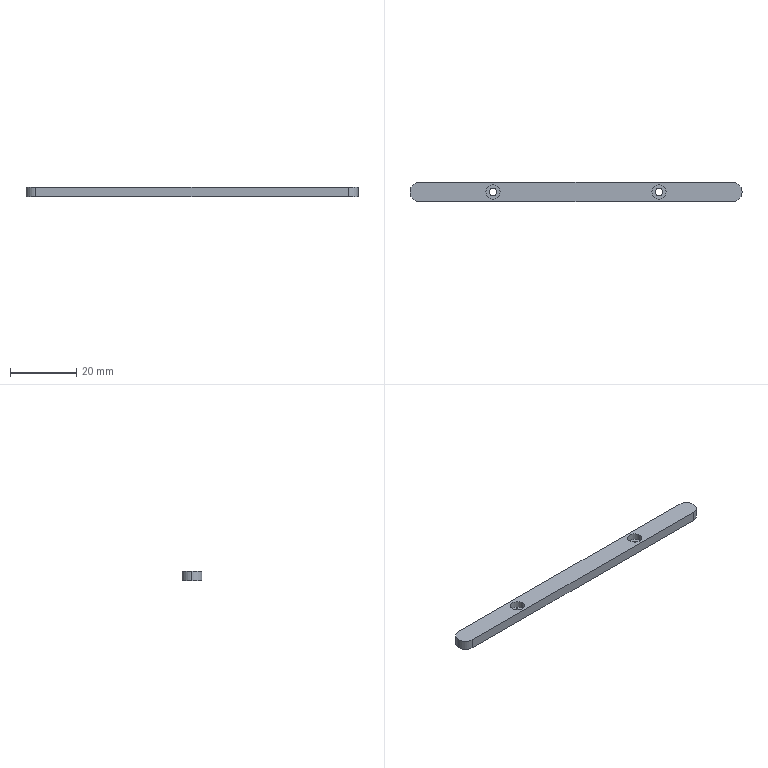Part | SolidWorks | features 3DProfileFeature 1, Extrusion 1, Fillet 1, HoleWzd 1 | 1 solid | 18 faces | box 100 x 6 x 3 mm | volume 1710 mm3 | cylinder 12 | plane 6 | commonest cylinder face diameters 2.4 x4 4.3 x4 6 x4
STEP:
#1=CARTESIAN_POINT('',(-27.15,-40.35,1.));
#2=VERTEX_POINT('',#1);
#3=CARTESIAN_POINT('',(-22.85,-40.35,1.));
#4=VERTEX_POINT('',#3);
#5=CARTESIAN_POINT('',(-25.,-40.35,1.));
#6=DIRECTION('',(0.,0.,1.));
#7=DIRECTION('',(1.,0.,0.));
#8=AXIS2_PLACEMENT_3D('',#5,#6,#7);
#9=CIRCLE('',#8,2.15);
#10=EDGE_CURVE('',#2,#4,#9,.T.);
#11=ORIENTED_EDGE('',*,*,#10,.F.);
#12=CARTESIAN_POINT('',(-27.15,-40.35,3.));
#13=VERTEX_POINT('',#12);
#14=CARTESIAN_POINT('',(-27.15,-40.35,3.));
#15=DIRECTION('',(0.,0.,1.));
#16=VECTOR('',#15,1000.);
#17=LINE('',#14,#16);
#18=EDGE_CURVE('',#2,#13,#17,.T.);
#19=ORIENTED_EDGE('',*,*,#18,.T.);
#20=CARTESIAN_POINT('',(-22.85,-40.35,3.));
#21=VERTEX_POINT('',#20);
#22=CARTESIAN_POINT('',(-25.,-40.35,3.));
#23=DIRECTION('',(0.,0.,1.));
#24=DIRECTION('',(1.,0.,0.));
#25=AXIS2_PLACEMENT_3D('',#22,#23,#24);
#26=CIRCLE('',#25,2.15);
#27=EDGE_CURVE('',#13,#21,#26,.T.);
#28=ORIENTED_EDGE('',*,*,#27,.T.);
#29=CARTESIAN_POINT('',(-22.85,-40.35,3.));
#30=DIRECTION('',(0.,0.,1.));
#31=VECTOR('',#30,1000.);
#32=LINE('',#29,#31);
#33=EDGE_CURVE('',#4,#21,#32,.T.);
#34=ORIENTED_EDGE('',*,*,#33,.F.);
#35=EDGE_LOOP('',(#11,#19,#28,#34));
#36=FACE_OUTER_BOUND('',#35,.T.);
#37=CARTESIAN_POINT('',(-25.,-40.35,3.));
#38=DIRECTION('',(0.,0.,1.));
#39=DIRECTION('',(1.,0.,0.));
#40=AXIS2_PLACEMENT_3D('',#37,#38,#39);
#41=CYLINDRICAL_SURFACE('',#40,2.15);
#42=ADVANCED_FACE('',(#36),#41,.F.);
#43=CARTESIAN_POINT('',(-26.2,-40.35,0.));
#44=VERTEX_POINT('',#43);
#45=CARTESIAN_POINT('',(-23.8,-40.35,0.));
#46=VERTEX_POINT('',#45);
#47=CARTESIAN_POINT('',(-25.,-40.35,0.));
#48=DIRECTION('',(0.,0.,1.));
#49=DIRECTION('',(1.,0.,0.));
#50=AXIS2_PLACEMENT_3D('',#47,#48,#49);
#51=CIRCLE('',#50,1.2);
#52=EDGE_CURVE('',#44,#46,#51,.T.);
#53=ORIENTED_EDGE('',*,*,#52,.F.);
#54=CARTESIAN_POINT('',(-26.2,-40.35,1.));
#55=VERTEX_POINT('',#54);
#56=CARTESIAN_POINT('',(-26.2,-40.35,3.));
#57=DIRECTION('',(0.,0.,1.));
#58=VECTOR('',#57,1000.);
#59=LINE('',#56,#58);
#60=EDGE_CURVE('',#44,#55,#59,.T.);
#61=ORIENTED_EDGE('',*,*,#60,.T.);
#62=CARTESIAN_POINT('',(-23.8,-40.35,1.));
#63=VERTEX_POINT('',#62);
#64=CARTESIAN_POINT('',(-25.,-40.35,1.));
#65=DIRECTION('',(0.,0.,1.));
#66=DIRECTION('',(1.,0.,0.));
#67=AXIS2_PLACEMENT_3D('',#64,#65,#66);
#68=CIRCLE('',#67,1.2);
#69=EDGE_CURVE('',#55,#63,#68,.T.);
#70=ORIENTED_EDGE('',*,*,#69,.T.);
#71=CARTESIAN_POINT('',(-23.8,-40.35,3.));
#72=DIRECTION('',(0.,0.,1.));
#73=VECTOR('',#72,1000.);
#74=LINE('',#71,#73);
#75=EDGE_CURVE('',#46,#63,#74,.T.);
#76=ORIENTED_EDGE('',*,*,#75,.F.);
#77=EDGE_LOOP('',(#53,#61,#70,#76));
#78=FACE_OUTER_BOUND('',#77,.T.);
#79=CARTESIAN_POINT('',(-25.,-40.35,3.));
#80=DIRECTION('',(0.,0.,1.));
#81=DIRECTION('',(1.,0.,0.));
#82=AXIS2_PLACEMENT_3D('',#79,#80,#81);
#83=CYLINDRICAL_SURFACE('',#82,1.2);
#84=ADVANCED_FACE('',(#78),#83,.F.);
#85=CARTESIAN_POINT('',(22.85,-40.35,1.));
#86=VERTEX_POINT('',#85);
#87=CARTESIAN_POINT('',(27.15,-40.35,1.));
#88=VERTEX_POINT('',#87);
#89=CARTESIAN_POINT('',(25.,-40.35,1.));
#90=DIRECTION('',(0.,0.,1.));
#91=DIRECTION('',(1.,0.,0.));
#92=AXIS2_PLACEMENT_3D('',#89,#90,#91);
#93=CIRCLE('',#92,2.15);
#94=EDGE_CURVE('',#86,#88,#93,.T.);
#95=ORIENTED_EDGE('',*,*,#94,.F.);
#96=CARTESIAN_POINT('',(22.85,-40.35,3.));
#97=VERTEX_POINT('',#96);
#98=CARTESIAN_POINT('',(22.85,-40.35,3.));
#99=DIRECTION('',(0.,0.,1.));
#100=VECTOR('',#99,1000.);
#101=LINE('',#98,#100);
#102=EDGE_CURVE('',#86,#97,#101,.T.);
#103=ORIENTED_EDGE('',*,*,#102,.T.);
#104=CARTESIAN_POINT('',(27.15,-40.35,3.));
#105=VERTEX_POINT('',#104);
#106=CARTESIAN_POINT('',(25.,-40.35,3.));
#107=DIRECTION('',(0.,0.,1.));
#108=DIRECTION('',(1.,0.,0.));
#109=AXIS2_PLACEMENT_3D('',#106,#107,#108);
#110=CIRCLE('',#109,2.15);
#111=EDGE_CURVE('',#97,#105,#110,.T.);
#112=ORIENTED_EDGE('',*,*,#111,.T.);
#113=CARTESIAN_POINT('',(27.15,-40.35,3.));
#114=DIRECTION('',(0.,0.,1.));
#115=VECTOR('',#114,1000.);
#116=LINE('',#113,#115);
#117=EDGE_CURVE('',#88,#105,#116,.T.);
#118=ORIENTED_EDGE('',*,*,#117,.F.);
#119=EDGE_LOOP('',(#95,#103,#112,#118));
#120=FACE_OUTER_BOUND('',#119,.T.);
#121=CARTESIAN_POINT('',(25.,-40.35,3.));
#122=DIRECTION('',(0.,0.,1.));
#123=DIRECTION('',(1.,0.,0.));
#124=AXIS2_PLACEMENT_3D('',#121,#122,#123);
#125=CYLINDRICAL_SURFACE('',#124,2.15);
#126=ADVANCED_FACE('',(#120),#125,.F.);
#127=CARTESIAN_POINT('',(23.8,-40.35,0.));
#128=VERTEX_POINT('',#127);
#129=CARTESIAN_POINT('',(26.2,-40.35,0.));
#130=VERTEX_POINT('',#129);
#131=CARTESIAN_POINT('',(25.,-40.35,0.));
#132=DIRECTION('',(0.,0.,1.));
#133=DIRECTION('',(1.,0.,0.));
#134=AXIS2_PLACEMENT_3D('',#131,#132,#133);
#135=CIRCLE('',#134,1.2);
#136=EDGE_CURVE('',#128,#130,#135,.T.);
#137=ORIENTED_EDGE('',*,*,#136,.F.);
#138=CARTESIAN_POINT('',(23.8,-40.35,1.));
#139=VERTEX_POINT('',#138);
#140=CARTESIAN_POINT('',(23.8,-40.35,3.));
#141=DIRECTION('',(0.,0.,1.));
#142=VECTOR('',#141,1000.);
#143=LINE('',#140,#142);
#144=EDGE_CURVE('',#128,#139,#143,.T.);
#145=ORIENTED_EDGE('',*,*,#144,.T.);
#146=CARTESIAN_POINT('',(26.2,-40.35,1.));
#147=VERTEX_POINT('',#146);
#148=CARTESIAN_POINT('',(25.,-40.35,1.));
#149=DIRECTION('',(0.,0.,1.));
#150=DIRECTION('',(1.,0.,0.));
#151=AXIS2_PLACEMENT_3D('',#148,#149,#150);
#152=CIRCLE('',#151,1.2);
#153=EDGE_CURVE('',#139,#147,#152,.T.);
#154=ORIENTED_EDGE('',*,*,#153,.T.);
#155=CARTESIAN_POINT('',(26.2,-40.35,3.));
#156=DIRECTION('',(0.,0.,1.));
#157=VECTOR('',#156,1000.);
#158=LINE('',#155,#157);
#159=EDGE_CURVE('',#130,#147,#158,.T.);
#160=ORIENTED_EDGE('',*,*,#159,.F.);
#161=EDGE_LOOP('',(#137,#145,#154,#160));
#162=FACE_OUTER_BOUND('',#161,.T.);
#163=CARTESIAN_POINT('',(25.,-40.35,3.));
#164=DIRECTION('',(0.,0.,1.));
#165=DIRECTION('',(1.,0.,0.));
#166=AXIS2_PLACEMENT_3D('',#163,#164,#165);
#167=CYLINDRICAL_SURFACE('',#166,1.2);
#168=ADVANCED_FACE('',(#162),#167,.F.);
#169=CARTESIAN_POINT('',(-47.,-43.35,0.));
#170=VERTEX_POINT('',#169);
#171=CARTESIAN_POINT('',(47.,-43.35,0.));
#172=VERTEX_POINT('',#171);
#173=CARTESIAN_POINT('',(-50.,-43.35,0.));
#174=DIRECTION('',(1.,0.,0.));
#175=VECTOR('',#174,1000.);
#176=LINE('',#173,#175);
#177=EDGE_CURVE('',#170,#172,#176,.T.);
#178=ORIENTED_EDGE('',*,*,#177,.T.);
#179=CARTESIAN_POINT('',(47.,-43.35,3.));
#180=VERTEX_POINT('',#179);
#181=CARTESIAN_POINT('',(47.,-43.35,3.));
#182=DIRECTION('',(0.,0.,1.));
#183=VECTOR('',#182,1000.);
#184=LINE('',#181,#183);
#185=EDGE_CURVE('',#172,#180,#184,.T.);
#186=ORIENTED_EDGE('',*,*,#185,.T.);
#187=CARTESIAN_POINT('',(-47.,-43.35,3.));
#188=VERTEX_POINT('',#187);
#189=CARTESIAN_POINT('',(-50.,-43.35,3.));
#190=DIRECTION('',(1.,0.,0.));
#191=VECTOR('',#190,1000.);
#192=LINE('',#189,#191);
#193=EDGE_CURVE('',#188,#180,#192,.T.);
#194=ORIENTED_EDGE('',*,*,#193,.F.);
#195=CARTESIAN_POINT('',(-47.,-43.35,3.));
#196=DIRECTION('',(0.,0.,-1.));
#197=VECTOR('',#196,1000.);
#198=LINE('',#195,#197);
#199=EDGE_CURVE('',#188,#170,#198,.T.);
#200=ORIENTED_EDGE('',*,*,#199,.T.);
#201=EDGE_LOOP('',(#178,#186,#194,#200));
#202=FACE_OUTER_BOUND('',#201,.T.);
#203=CARTESIAN_POINT('',(-50.,-43.35,3.));
#204=DIRECTION('',(0.,1.,0.));
#205=DIRECTION('',(-1.,0.,0.));
#206=AXIS2_PLACEMENT_3D('',#203,#204,#205);
#207=PLANE('',#206);
#208=ADVANCED_FACE('',(#202),#207,.F.);
#209=CARTESIAN_POINT('',(-47.,-37.35,3.));
#210=VERTEX_POINT('',#209);
#211=CARTESIAN_POINT('',(47.,-37.35,3.));
#212=VERTEX_POINT('',#211);
#213=CARTESIAN_POINT('',(-50.,-37.35,3.));
#214=DIRECTION('',(1.,0.,0.));
#215=VECTOR('',#214,1000.);
#216=LINE('',#213,#215);
#217=EDGE_CURVE('',#210,#212,#216,.T.);
#218=ORIENTED_EDGE('',*,*,#217,.T.);
#219=CARTESIAN_POINT('',(47.,-37.35,0.));
#220=VERTEX_POINT('',#219);
#221=CARTESIAN_POINT('',(47.,-37.35,3.));
#222=DIRECTION('',(0.,0.,-1.));
#223=VECTOR('',#222,1000.);
#224=LINE('',#221,#223);
#225=EDGE_CURVE('',#212,#220,#224,.T.);
#226=ORIENTED_EDGE('',*,*,#225,.T.);
#227=CARTESIAN_POINT('',(-47.,-37.35,0.));
#228=VERTEX_POINT('',#227);
#229=CARTESIAN_POINT('',(-50.,-37.35,0.));
#230=DIRECTION('',(1.,0.,0.));
#231=VECTOR('',#230,1000.);
#232=LINE('',#229,#231);
#233=EDGE_CURVE('',#228,#220,#232,.T.);
#234=ORIENTED_EDGE('',*,*,#233,.F.);
#235=CARTESIAN_POINT('',(-47.,-37.35,3.));
#236=DIRECTION('',(0.,0.,1.));
#237=VECTOR('',#236,1000.);
#238=LINE('',#235,#237);
#239=EDGE_CURVE('',#228,#210,#238,.T.);
#240=ORIENTED_EDGE('',*,*,#239,.T.);
#241=EDGE_LOOP('',(#218,#226,#234,#240));
#242=FACE_OUTER_BOUND('',#241,.T.);
#243=CARTESIAN_POINT('',(-50.,-37.35,3.));
#244=DIRECTION('',(0.,1.,0.));
#245=DIRECTION('',(-1.,0.,0.));
#246=AXIS2_PLACEMENT_3D('',#243,#244,#245);
#247=PLANE('',#246);
#248=ADVANCED_FACE('',(#242),#247,.T.);
#249=CARTESIAN_POINT('',(-25.,-40.35,3.));
#250=DIRECTION('',(0.,0.,1.));
#251=DIRECTION('',(1.,0.,0.));
#252=AXIS2_PLACEMENT_3D('',#249,#250,#251);
#253=CIRCLE('',#252,2.15);
#254=EDGE_CURVE('',#21,#13,#253,.T.);
#255=ORIENTED_EDGE('',*,*,#254,.F.);
#256=ORIENTED_EDGE('',*,*,#27,.F.);
#257=EDGE_LOOP('',(#255,#256));
#258=FACE_BOUND('',#257,.T.);
#259=CARTESIAN_POINT('',(25.,-40.35,3.));
#260=DIRECTION('',(0.,0.,1.));
#261=DIRECTION('',(1.,0.,0.));
#262=AXIS2_PLACEMENT_3D('',#259,#260,#261);
#263=CIRCLE('',#262,2.15);
#264=EDGE_CURVE('',#105,#97,#263,.T.);
#265=ORIENTED_EDGE('',*,*,#264,.F.);
#266=ORIENTED_EDGE('',*,*,#111,.F.);
#267=EDGE_LOOP('',(#265,#266));
#268=FACE_BOUND('',#267,.T.);
#269=CARTESIAN_POINT('',(50.,-40.35,3.));
#270=VERTEX_POINT('',#269);
#271=CARTESIAN_POINT('',(47.,-40.35,3.));
#272=DIRECTION('',(0.,0.,1.));
#273=DIRECTION('',(1.,0.,0.));
#274=AXIS2_PLACEMENT_3D('',#271,#272,#273);
#275=CIRCLE('',#274,3.);
#276=EDGE_CURVE('',#180,#270,#275,.T.);
#277=ORIENTED_EDGE('',*,*,#276,.T.);
#278=CARTESIAN_POINT('',(47.,-40.35,3.));
#279=DIRECTION('',(0.,0.,1.));
#280=DIRECTION('',(1.,0.,0.));
#281=AXIS2_PLACEMENT_3D('',#278,#279,#280);
#282=CIRCLE('',#281,3.);
#283=EDGE_CURVE('',#270,#212,#282,.T.);
#284=ORIENTED_EDGE('',*,*,#283,.T.);
#285=ORIENTED_EDGE('',*,*,#217,.F.);
#286=CARTESIAN_POINT('',(-50.,-40.35,3.));
#287=VERTEX_POINT('',#286);
#288=CARTESIAN_POINT('',(-47.,-40.35,3.));
#289=DIRECTION('',(0.,0.,1.));
#290=DIRECTION('',(1.,0.,0.));
#291=AXIS2_PLACEMENT_3D('',#288,#289,#290);
#292=CIRCLE('',#291,3.);
#293=EDGE_CURVE('',#210,#287,#292,.T.);
#294=ORIENTED_EDGE('',*,*,#293,.T.);
#295=CARTESIAN_POINT('',(-47.,-40.35,3.));
#296=DIRECTION('',(0.,0.,1.));
#297=DIRECTION('',(1.,0.,0.));
#298=AXIS2_PLACEMENT_3D('',#295,#296,#297);
#299=CIRCLE('',#298,3.);
#300=EDGE_CURVE('',#287,#188,#299,.T.);
#301=ORIENTED_EDGE('',*,*,#300,.T.);
#302=ORIENTED_EDGE('',*,*,#193,.T.);
#303=EDGE_LOOP('',(#277,#284,#285,#294,#301,#302));
#304=FACE_OUTER_BOUND('',#303,.T.);
#305=CARTESIAN_POINT('',(0.,0.,3.));
#306=DIRECTION('',(0.,0.,1.));
#307=DIRECTION('',(1.,0.,0.));
#308=AXIS2_PLACEMENT_3D('',#305,#306,#307);
#309=PLANE('',#308);
#310=ADVANCED_FACE('',(#258,#268,#304),#309,.T.);
#311=CARTESIAN_POINT('',(-25.,-40.35,0.));
#312=DIRECTION('',(0.,0.,1.));
#313=DIRECTION('',(1.,0.,0.));
#314=AXIS2_PLACEMENT_3D('',#311,#312,#313);
#315=CIRCLE('',#314,1.2);
#316=EDGE_CURVE('',#46,#44,#315,.T.);
#317=ORIENTED_EDGE('',*,*,#316,.T.);
#318=ORIENTED_EDGE('',*,*,#52,.T.);
#319=EDGE_LOOP('',(#317,#318));
#320=FACE_BOUND('',#319,.T.);
#321=CARTESIAN_POINT('',(25.,-40.35,0.));
#322=DIRECTION('',(0.,0.,1.));
#323=DIRECTION('',(1.,0.,0.));
#324=AXIS2_PLACEMENT_3D('',#321,#322,#323);
#325=CIRCLE('',#324,1.2);
#326=EDGE_CURVE('',#130,#128,#325,.T.);
#327=ORIENTED_EDGE('',*,*,#326,.T.);
#328=ORIENTED_EDGE('',*,*,#136,.T.);
#329=EDGE_LOOP('',(#327,#328));
#330=FACE_BOUND('',#329,.T.);
#331=ORIENTED_EDGE('',*,*,#233,.T.);
#332=CARTESIAN_POINT('',(50.,-40.35,0.));
#333=VERTEX_POINT('',#332);
#334=CARTESIAN_POINT('',(47.,-40.35,0.));
#335=DIRECTION('',(0.,0.,-1.));
#336=DIRECTION('',(1.,0.,0.));
#337=AXIS2_PLACEMENT_3D('',#334,#335,#336);
#338=CIRCLE('',#337,3.);
#339=EDGE_CURVE('',#220,#333,#338,.T.);
#340=ORIENTED_EDGE('',*,*,#339,.T.);
#341=CARTESIAN_POINT('',(47.,-40.35,0.));
#342=DIRECTION('',(0.,0.,-1.));
#343=DIRECTION('',(1.,0.,0.));
#344=AXIS2_PLACEMENT_3D('',#341,#342,#343);
#345=CIRCLE('',#344,3.);
#346=EDGE_CURVE('',#333,#172,#345,.T.);
#347=ORIENTED_EDGE('',*,*,#346,.T.);
#348=ORIENTED_EDGE('',*,*,#177,.F.);
#349=CARTESIAN_POINT('',(-50.,-40.35,0.));
#350=VERTEX_POINT('',#349);
#351=CARTESIAN_POINT('',(-47.,-40.35,0.));
#352=DIRECTION('',(0.,0.,-1.));
#353=DIRECTION('',(1.,0.,0.));
#354=AXIS2_PLACEMENT_3D('',#351,#352,#353);
#355=CIRCLE('',#354,3.);
#356=EDGE_CURVE('',#170,#350,#355,.T.);
#357=ORIENTED_EDGE('',*,*,#356,.T.);
#358=CARTESIAN_POINT('',(-47.,-40.35,0.));
#359=DIRECTION('',(0.,0.,-1.));
#360=DIRECTION('',(1.,0.,0.));
#361=AXIS2_PLACEMENT_3D('',#358,#359,#360);
#362=CIRCLE('',#361,3.);
#363=EDGE_CURVE('',#350,#228,#362,.T.);
#364=ORIENTED_EDGE('',*,*,#363,.T.);
#365=EDGE_LOOP('',(#331,#340,#347,#348,#357,#364));
#366=FACE_OUTER_BOUND('',#365,.T.);
#367=CARTESIAN_POINT('',(0.,0.,0.));
#368=DIRECTION('',(0.,0.,1.));
#369=DIRECTION('',(1.,0.,0.));
#370=AXIS2_PLACEMENT_3D('',#367,#368,#369);
#371=PLANE('',#370);
#372=ADVANCED_FACE('',(#320,#330,#366),#371,.F.);
#373=CARTESIAN_POINT('',(50.,-40.35,0.));
#374=DIRECTION('',(0.,0.,-1.));
#375=VECTOR('',#374,1000.);
#376=LINE('',#373,#375);
#377=EDGE_CURVE('',#270,#333,#376,.T.);
#378=ORIENTED_EDGE('',*,*,#377,.F.);
#379=ORIENTED_EDGE('',*,*,#276,.F.);
#380=ORIENTED_EDGE('',*,*,#185,.F.);
#381=ORIENTED_EDGE('',*,*,#346,.F.);
#382=EDGE_LOOP('',(#378,#379,#380,#381));
#383=FACE_OUTER_BOUND('',#382,.T.);
#384=CARTESIAN_POINT('',(47.,-40.35,3.));
#385=DIRECTION('',(0.,0.,1.));
#386=DIRECTION('',(1.,0.,0.));
#387=AXIS2_PLACEMENT_3D('',#384,#385,#386);
#388=CYLINDRICAL_SURFACE('',#387,3.);
#389=ADVANCED_FACE('',(#383),#388,.T.);
#390=ORIENTED_EDGE('',*,*,#283,.F.);
#391=ORIENTED_EDGE('',*,*,#377,.T.);
#392=ORIENTED_EDGE('',*,*,#339,.F.);
#393=ORIENTED_EDGE('',*,*,#225,.F.);
#394=EDGE_LOOP('',(#390,#391,#392,#393));
#395=FACE_OUTER_BOUND('',#394,.T.);
#396=CARTESIAN_POINT('',(47.,-40.35,3.));
#397=DIRECTION('',(0.,0.,-1.));
#398=DIRECTION('',(-1.,0.,0.));
#399=AXIS2_PLACEMENT_3D('',#396,#397,#398);
#400=CYLINDRICAL_SURFACE('',#399,3.);
#401=ADVANCED_FACE('',(#395),#400,.T.);
#402=ORIENTED_EDGE('',*,*,#199,.F.);
#403=ORIENTED_EDGE('',*,*,#300,.F.);
#404=CARTESIAN_POINT('',(-50.,-40.35,3.));
#405=DIRECTION('',(0.,0.,1.));
#406=VECTOR('',#405,1000.);
#407=LINE('',#404,#406);
#408=EDGE_CURVE('',#350,#287,#407,.T.);
#409=ORIENTED_EDGE('',*,*,#408,.F.);
#410=ORIENTED_EDGE('',*,*,#356,.F.);
#411=EDGE_LOOP('',(#402,#403,#409,#410));
#412=FACE_OUTER_BOUND('',#411,.T.);
#413=CARTESIAN_POINT('',(-47.,-40.35,3.));
#414=DIRECTION('',(0.,0.,-1.));
#415=DIRECTION('',(-1.,0.,0.));
#416=AXIS2_PLACEMENT_3D('',#413,#414,#415);
#417=CYLINDRICAL_SURFACE('',#416,3.);
#418=ADVANCED_FACE('',(#412),#417,.T.);
#419=ORIENTED_EDGE('',*,*,#293,.F.);
#420=ORIENTED_EDGE('',*,*,#239,.F.);
#421=ORIENTED_EDGE('',*,*,#363,.F.);
#422=ORIENTED_EDGE('',*,*,#408,.T.);
#423=EDGE_LOOP('',(#419,#420,#421,#422));
#424=FACE_OUTER_BOUND('',#423,.T.);
#425=CARTESIAN_POINT('',(-47.,-40.35,3.));
#426=DIRECTION('',(0.,0.,1.));
#427=DIRECTION('',(1.,0.,0.));
#428=AXIS2_PLACEMENT_3D('',#425,#426,#427);
#429=CYLINDRICAL_SURFACE('',#428,3.);
#430=ADVANCED_FACE('',(#424),#429,.T.);
#431=ORIENTED_EDGE('',*,*,#144,.F.);
#432=ORIENTED_EDGE('',*,*,#326,.F.);
#433=ORIENTED_EDGE('',*,*,#159,.T.);
#434=CARTESIAN_POINT('',(25.,-40.35,1.));
#435=DIRECTION('',(0.,0.,1.));
#436=DIRECTION('',(1.,0.,0.));
#437=AXIS2_PLACEMENT_3D('',#434,#435,#436);
#438=CIRCLE('',#437,1.2);
#439=EDGE_CURVE('',#147,#139,#438,.T.);
#440=ORIENTED_EDGE('',*,*,#439,.T.);
#441=EDGE_LOOP('',(#431,#432,#433,#440));
#442=FACE_OUTER_BOUND('',#441,.T.);
#443=CARTESIAN_POINT('',(25.,-40.35,3.));
#444=DIRECTION('',(0.,0.,1.));
#445=DIRECTION('',(1.,0.,0.));
#446=AXIS2_PLACEMENT_3D('',#443,#444,#445);
#447=CYLINDRICAL_SURFACE('',#446,1.2);
#448=ADVANCED_FACE('',(#442),#447,.F.);
#449=ORIENTED_EDGE('',*,*,#439,.F.);
#450=ORIENTED_EDGE('',*,*,#153,.F.);
#451=EDGE_LOOP('',(#449,#450));
#452=FACE_BOUND('',#451,.T.);
#453=CARTESIAN_POINT('',(25.,-40.35,1.));
#454=DIRECTION('',(0.,0.,1.));
#455=DIRECTION('',(1.,0.,0.));
#456=AXIS2_PLACEMENT_3D('',#453,#454,#455);
#457=CIRCLE('',#456,2.15);
#458=EDGE_CURVE('',#88,#86,#457,.T.);
#459=ORIENTED_EDGE('',*,*,#458,.T.);
#460=ORIENTED_EDGE('',*,*,#94,.T.);
#461=EDGE_LOOP('',(#459,#460));
#462=FACE_OUTER_BOUND('',#461,.T.);
#463=CARTESIAN_POINT('',(26.2,-40.35,1.));
#464=DIRECTION('',(0.,0.,-1.));
#465=DIRECTION('',(-1.,0.,0.));
#466=AXIS2_PLACEMENT_3D('',#463,#464,#465);
#467=PLANE('',#466);
#468=ADVANCED_FACE('',(#452,#462),#467,.F.);
#469=ORIENTED_EDGE('',*,*,#102,.F.);
#470=ORIENTED_EDGE('',*,*,#458,.F.);
#471=ORIENTED_EDGE('',*,*,#117,.T.);
#472=ORIENTED_EDGE('',*,*,#264,.T.);
#473=EDGE_LOOP('',(#469,#470,#471,#472));
#474=FACE_OUTER_BOUND('',#473,.T.);
#475=CARTESIAN_POINT('',(25.,-40.35,3.));
#476=DIRECTION('',(0.,0.,1.));
#477=DIRECTION('',(1.,0.,0.));
#478=AXIS2_PLACEMENT_3D('',#475,#476,#477);
#479=CYLINDRICAL_SURFACE('',#478,2.15);
#480=ADVANCED_FACE('',(#474),#479,.F.);
#481=ORIENTED_EDGE('',*,*,#60,.F.);
#482=ORIENTED_EDGE('',*,*,#316,.F.);
#483=ORIENTED_EDGE('',*,*,#75,.T.);
#484=CARTESIAN_POINT('',(-25.,-40.35,1.));
#485=DIRECTION('',(0.,0.,1.));
#486=DIRECTION('',(1.,0.,0.));
#487=AXIS2_PLACEMENT_3D('',#484,#485,#486);
#488=CIRCLE('',#487,1.2);
#489=EDGE_CURVE('',#63,#55,#488,.T.);
#490=ORIENTED_EDGE('',*,*,#489,.T.);
#491=EDGE_LOOP('',(#481,#482,#483,#490));
#492=FACE_OUTER_BOUND('',#491,.T.);
#493=CARTESIAN_POINT('',(-25.,-40.35,3.));
#494=DIRECTION('',(0.,0.,1.));
#495=DIRECTION('',(1.,0.,0.));
#496=AXIS2_PLACEMENT_3D('',#493,#494,#495);
#497=CYLINDRICAL_SURFACE('',#496,1.2);
#498=ADVANCED_FACE('',(#492),#497,.F.);
#499=ORIENTED_EDGE('',*,*,#489,.F.);
#500=ORIENTED_EDGE('',*,*,#69,.F.);
#501=EDGE_LOOP('',(#499,#500));
#502=FACE_BOUND('',#501,.T.);
#503=CARTESIAN_POINT('',(-25.,-40.35,1.));
#504=DIRECTION('',(0.,0.,1.));
#505=DIRECTION('',(1.,0.,0.));
#506=AXIS2_PLACEMENT_3D('',#503,#504,#505);
#507=CIRCLE('',#506,2.15);
#508=EDGE_CURVE('',#4,#2,#507,.T.);
#509=ORIENTED_EDGE('',*,*,#508,.T.);
#510=ORIENTED_EDGE('',*,*,#10,.T.);
#511=EDGE_LOOP('',(#509,#510));
#512=FACE_OUTER_BOUND('',#511,.T.);
#513=CARTESIAN_POINT('',(-23.8,-40.35,1.));
#514=DIRECTION('',(0.,0.,-1.));
#515=DIRECTION('',(-1.,0.,0.));
#516=AXIS2_PLACEMENT_3D('',#513,#514,#515);
#517=PLANE('',#516);
#518=ADVANCED_FACE('',(#502,#512),#517,.F.);
#519=ORIENTED_EDGE('',*,*,#18,.F.);
#520=ORIENTED_EDGE('',*,*,#508,.F.);
#521=ORIENTED_EDGE('',*,*,#33,.T.);
#522=ORIENTED_EDGE('',*,*,#254,.T.);
#523=EDGE_LOOP('',(#519,#520,#521,#522));
#524=FACE_OUTER_BOUND('',#523,.T.);
#525=CARTESIAN_POINT('',(-25.,-40.35,3.));
#526=DIRECTION('',(0.,0.,1.));
#527=DIRECTION('',(1.,0.,0.));
#528=AXIS2_PLACEMENT_3D('',#525,#526,#527);
#529=CYLINDRICAL_SURFACE('',#528,2.15);
#530=ADVANCED_FACE('',(#524),#529,.F.);
#531=CLOSED_SHELL('',(#42,#84,#126,#168,#208,#248,#310,#372,#389,#401,#418,#430,#448,#468,#480,#498,#518,#530));
#532=MANIFOLD_SOLID_BREP('',#531);
#533=CARTESIAN_POINT('',(0.,0.,0.));
#534=DIRECTION('',(0.,0.,1.));
#535=DIRECTION('',(1.,0.,0.));
#536=AXIS2_PLACEMENT_3D('',#533,#534,#535);
#537=(LENGTH_UNIT()NAMED_UNIT(*)SI_UNIT(.MILLI.,.METRE.));
#538=UNCERTAINTY_MEASURE_WITH_UNIT(LENGTH_MEASURE(0.00001),#537,'','');
#539=(NAMED_UNIT(*)PLANE_ANGLE_UNIT()SI_UNIT($,.RADIAN.));
#540=(NAMED_UNIT(*)SI_UNIT($,.STERADIAN.)SOLID_ANGLE_UNIT());
#541=(GEOMETRIC_REPRESENTATION_CONTEXT(3)GLOBAL_UNCERTAINTY_ASSIGNED_CONTEXT((#538))GLOBAL_UNIT_ASSIGNED_CONTEXT((#537,#539,#540))REPRESENTATION_CONTEXT('',''));
#542=ADVANCED_BREP_SHAPE_REPRESENTATION('',(#532,#536),#541);